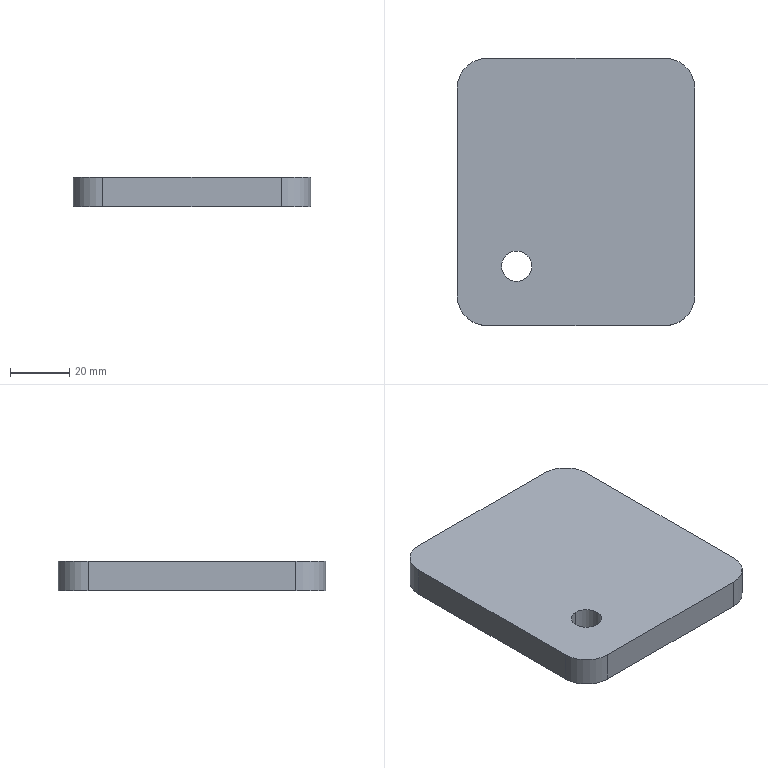Part | SolidWorks | features BaseBody 1 | 1 solid | 12 faces | box 80 x 90 x 10 mm | volume 70324 mm3 | cylinder 6 | plane 6 | commonest cylinder face diameters 20 x4 10.2 x2
STEP:
#1=CARTESIAN_POINT('',(-20.,-30.1,-5.));
#2=VERTEX_POINT('',#1);
#3=CARTESIAN_POINT('',(-20.,-19.9,-5.));
#4=VERTEX_POINT('',#3);
#5=CARTESIAN_POINT('',(-20.,-25.,-5.));
#6=DIRECTION('',(0.,0.,-1.));
#7=DIRECTION('',(0.,-1.,0.));
#8=AXIS2_PLACEMENT_3D('',#5,#6,#7);
#9=CIRCLE('',#8,5.1);
#10=EDGE_CURVE('',#2,#4,#9,.T.);
#11=ORIENTED_EDGE('',*,*,#10,.T.);
#12=CARTESIAN_POINT('',(-20.,-19.9,5.));
#13=VERTEX_POINT('',#12);
#14=CARTESIAN_POINT('',(-20.,-19.9,-5.));
#15=DIRECTION('',(0.,0.,1.));
#16=VECTOR('',#15,1000.);
#17=LINE('',#14,#16);
#18=EDGE_CURVE('',#4,#13,#17,.T.);
#19=ORIENTED_EDGE('',*,*,#18,.T.);
#20=CARTESIAN_POINT('',(-20.,-30.1,5.));
#21=VERTEX_POINT('',#20);
#22=CARTESIAN_POINT('',(-20.,-25.,5.));
#23=DIRECTION('',(0.,0.,1.));
#24=DIRECTION('',(0.,-1.,0.));
#25=AXIS2_PLACEMENT_3D('',#22,#23,#24);
#26=CIRCLE('',#25,5.1);
#27=EDGE_CURVE('',#13,#21,#26,.T.);
#28=ORIENTED_EDGE('',*,*,#27,.T.);
#29=CARTESIAN_POINT('',(-20.,-30.1,-5.));
#30=DIRECTION('',(0.,0.,1.));
#31=VECTOR('',#30,1000.);
#32=LINE('',#29,#31);
#33=EDGE_CURVE('',#2,#21,#32,.T.);
#34=ORIENTED_EDGE('',*,*,#33,.F.);
#35=EDGE_LOOP('',(#11,#19,#28,#34));
#36=FACE_OUTER_BOUND('',#35,.T.);
#37=CARTESIAN_POINT('',(-20.,-25.,-5.));
#38=DIRECTION('',(0.,0.,1.));
#39=DIRECTION('',(0.,-1.,0.));
#40=AXIS2_PLACEMENT_3D('',#37,#38,#39);
#41=CYLINDRICAL_SURFACE('',#40,5.1);
#42=ADVANCED_FACE('',(#36),#41,.F.);
#43=ORIENTED_EDGE('',*,*,#18,.F.);
#44=CARTESIAN_POINT('',(-20.,-25.,-5.));
#45=DIRECTION('',(0.,0.,-1.));
#46=DIRECTION('',(0.,-1.,0.));
#47=AXIS2_PLACEMENT_3D('',#44,#45,#46);
#48=CIRCLE('',#47,5.1);
#49=EDGE_CURVE('',#4,#2,#48,.T.);
#50=ORIENTED_EDGE('',*,*,#49,.T.);
#51=ORIENTED_EDGE('',*,*,#33,.T.);
#52=CARTESIAN_POINT('',(-20.,-25.,5.));
#53=DIRECTION('',(0.,0.,1.));
#54=DIRECTION('',(0.,-1.,0.));
#55=AXIS2_PLACEMENT_3D('',#52,#53,#54);
#56=CIRCLE('',#55,5.1);
#57=EDGE_CURVE('',#21,#13,#56,.T.);
#58=ORIENTED_EDGE('',*,*,#57,.T.);
#59=EDGE_LOOP('',(#43,#50,#51,#58));
#60=FACE_OUTER_BOUND('',#59,.T.);
#61=CARTESIAN_POINT('',(-20.,-25.,-5.));
#62=DIRECTION('',(0.,0.,1.));
#63=DIRECTION('',(0.,-1.,0.));
#64=AXIS2_PLACEMENT_3D('',#61,#62,#63);
#65=CYLINDRICAL_SURFACE('',#64,5.1);
#66=ADVANCED_FACE('',(#60),#65,.F.);
#67=ORIENTED_EDGE('',*,*,#57,.F.);
#68=ORIENTED_EDGE('',*,*,#27,.F.);
#69=EDGE_LOOP('',(#67,#68));
#70=FACE_BOUND('',#69,.T.);
#71=CARTESIAN_POINT('',(40.,-35.,5.));
#72=VERTEX_POINT('',#71);
#73=CARTESIAN_POINT('',(30.,-45.,5.));
#74=VERTEX_POINT('',#73);
#75=CARTESIAN_POINT('',(30.,-35.,5.));
#76=DIRECTION('',(0.,0.,-1.));
#77=DIRECTION('',(0.,1.,0.));
#78=AXIS2_PLACEMENT_3D('',#75,#76,#77);
#79=CIRCLE('',#78,10.);
#80=EDGE_CURVE('',#72,#74,#79,.T.);
#81=ORIENTED_EDGE('',*,*,#80,.F.);
#82=CARTESIAN_POINT('',(40.,35.,5.));
#83=VERTEX_POINT('',#82);
#84=CARTESIAN_POINT('',(40.,0.,5.));
#85=DIRECTION('',(0.,-1.,0.));
#86=VECTOR('',#85,1000.);
#87=LINE('',#84,#86);
#88=EDGE_CURVE('',#83,#72,#87,.T.);
#89=ORIENTED_EDGE('',*,*,#88,.F.);
#90=CARTESIAN_POINT('',(30.,45.,5.));
#91=VERTEX_POINT('',#90);
#92=CARTESIAN_POINT('',(30.,35.,5.));
#93=DIRECTION('',(0.,0.,-1.));
#94=DIRECTION('',(0.,1.,0.));
#95=AXIS2_PLACEMENT_3D('',#92,#93,#94);
#96=CIRCLE('',#95,10.);
#97=EDGE_CURVE('',#91,#83,#96,.T.);
#98=ORIENTED_EDGE('',*,*,#97,.F.);
#99=CARTESIAN_POINT('',(-30.,45.,5.));
#100=VERTEX_POINT('',#99);
#101=CARTESIAN_POINT('',(0.,45.,5.));
#102=DIRECTION('',(1.,0.,0.));
#103=VECTOR('',#102,1000.);
#104=LINE('',#101,#103);
#105=EDGE_CURVE('',#100,#91,#104,.T.);
#106=ORIENTED_EDGE('',*,*,#105,.F.);
#107=CARTESIAN_POINT('',(-40.,35.,5.));
#108=VERTEX_POINT('',#107);
#109=CARTESIAN_POINT('',(-30.,35.,5.));
#110=DIRECTION('',(0.,0.,-1.));
#111=DIRECTION('',(0.,1.,0.));
#112=AXIS2_PLACEMENT_3D('',#109,#110,#111);
#113=CIRCLE('',#112,10.);
#114=EDGE_CURVE('',#108,#100,#113,.T.);
#115=ORIENTED_EDGE('',*,*,#114,.F.);
#116=CARTESIAN_POINT('',(-40.,-35.,5.));
#117=VERTEX_POINT('',#116);
#118=CARTESIAN_POINT('',(-40.,0.,5.));
#119=DIRECTION('',(0.,1.,0.));
#120=VECTOR('',#119,1000.);
#121=LINE('',#118,#120);
#122=EDGE_CURVE('',#117,#108,#121,.T.);
#123=ORIENTED_EDGE('',*,*,#122,.F.);
#124=CARTESIAN_POINT('',(-30.,-45.,5.));
#125=VERTEX_POINT('',#124);
#126=CARTESIAN_POINT('',(-30.,-35.,5.));
#127=DIRECTION('',(0.,0.,-1.));
#128=DIRECTION('',(0.,1.,0.));
#129=AXIS2_PLACEMENT_3D('',#126,#127,#128);
#130=CIRCLE('',#129,10.);
#131=EDGE_CURVE('',#125,#117,#130,.T.);
#132=ORIENTED_EDGE('',*,*,#131,.F.);
#133=CARTESIAN_POINT('',(0.,-45.,5.));
#134=DIRECTION('',(-1.,0.,0.));
#135=VECTOR('',#134,1000.);
#136=LINE('',#133,#135);
#137=EDGE_CURVE('',#74,#125,#136,.T.);
#138=ORIENTED_EDGE('',*,*,#137,.F.);
#139=EDGE_LOOP('',(#81,#89,#98,#106,#115,#123,#132,#138));
#140=FACE_OUTER_BOUND('',#139,.T.);
#141=CARTESIAN_POINT('',(40.,-45.,5.));
#142=DIRECTION('',(0.,0.,-1.));
#143=DIRECTION('',(-1.,0.,0.));
#144=AXIS2_PLACEMENT_3D('',#141,#142,#143);
#145=PLANE('',#144);
#146=ADVANCED_FACE('',(#70,#140),#145,.F.);
#147=ORIENTED_EDGE('',*,*,#10,.F.);
#148=ORIENTED_EDGE('',*,*,#49,.F.);
#149=EDGE_LOOP('',(#147,#148));
#150=FACE_BOUND('',#149,.T.);
#151=CARTESIAN_POINT('',(-30.,45.,-5.));
#152=VERTEX_POINT('',#151);
#153=CARTESIAN_POINT('',(30.,45.,-5.));
#154=VERTEX_POINT('',#153);
#155=CARTESIAN_POINT('',(0.,45.,-5.));
#156=DIRECTION('',(1.,0.,0.));
#157=VECTOR('',#156,1000.);
#158=LINE('',#155,#157);
#159=EDGE_CURVE('',#152,#154,#158,.T.);
#160=ORIENTED_EDGE('',*,*,#159,.T.);
#161=CARTESIAN_POINT('',(40.,35.,-5.));
#162=VERTEX_POINT('',#161);
#163=CARTESIAN_POINT('',(30.,35.,-5.));
#164=DIRECTION('',(0.,0.,-1.));
#165=DIRECTION('',(0.,1.,0.));
#166=AXIS2_PLACEMENT_3D('',#163,#164,#165);
#167=CIRCLE('',#166,10.);
#168=EDGE_CURVE('',#154,#162,#167,.T.);
#169=ORIENTED_EDGE('',*,*,#168,.T.);
#170=CARTESIAN_POINT('',(40.,-35.,-5.));
#171=VERTEX_POINT('',#170);
#172=CARTESIAN_POINT('',(40.,0.,-5.));
#173=DIRECTION('',(0.,-1.,0.));
#174=VECTOR('',#173,1000.);
#175=LINE('',#172,#174);
#176=EDGE_CURVE('',#162,#171,#175,.T.);
#177=ORIENTED_EDGE('',*,*,#176,.T.);
#178=CARTESIAN_POINT('',(30.,-45.,-5.));
#179=VERTEX_POINT('',#178);
#180=CARTESIAN_POINT('',(30.,-35.,-5.));
#181=DIRECTION('',(0.,0.,-1.));
#182=DIRECTION('',(0.,1.,0.));
#183=AXIS2_PLACEMENT_3D('',#180,#181,#182);
#184=CIRCLE('',#183,10.);
#185=EDGE_CURVE('',#171,#179,#184,.T.);
#186=ORIENTED_EDGE('',*,*,#185,.T.);
#187=CARTESIAN_POINT('',(-30.,-45.,-5.));
#188=VERTEX_POINT('',#187);
#189=CARTESIAN_POINT('',(0.,-45.,-5.));
#190=DIRECTION('',(-1.,0.,0.));
#191=VECTOR('',#190,1000.);
#192=LINE('',#189,#191);
#193=EDGE_CURVE('',#179,#188,#192,.T.);
#194=ORIENTED_EDGE('',*,*,#193,.T.);
#195=CARTESIAN_POINT('',(-40.,-35.,-5.));
#196=VERTEX_POINT('',#195);
#197=CARTESIAN_POINT('',(-30.,-35.,-5.));
#198=DIRECTION('',(0.,0.,-1.));
#199=DIRECTION('',(0.,1.,0.));
#200=AXIS2_PLACEMENT_3D('',#197,#198,#199);
#201=CIRCLE('',#200,10.);
#202=EDGE_CURVE('',#188,#196,#201,.T.);
#203=ORIENTED_EDGE('',*,*,#202,.T.);
#204=CARTESIAN_POINT('',(-40.,35.,-5.));
#205=VERTEX_POINT('',#204);
#206=CARTESIAN_POINT('',(-40.,0.,-5.));
#207=DIRECTION('',(0.,1.,0.));
#208=VECTOR('',#207,1000.);
#209=LINE('',#206,#208);
#210=EDGE_CURVE('',#196,#205,#209,.T.);
#211=ORIENTED_EDGE('',*,*,#210,.T.);
#212=CARTESIAN_POINT('',(-30.,35.,-5.));
#213=DIRECTION('',(0.,0.,-1.));
#214=DIRECTION('',(0.,1.,0.));
#215=AXIS2_PLACEMENT_3D('',#212,#213,#214);
#216=CIRCLE('',#215,10.);
#217=EDGE_CURVE('',#205,#152,#216,.T.);
#218=ORIENTED_EDGE('',*,*,#217,.T.);
#219=EDGE_LOOP('',(#160,#169,#177,#186,#194,#203,#211,#218));
#220=FACE_OUTER_BOUND('',#219,.T.);
#221=CARTESIAN_POINT('',(40.,-45.,-5.));
#222=DIRECTION('',(0.,0.,-1.));
#223=DIRECTION('',(-1.,0.,0.));
#224=AXIS2_PLACEMENT_3D('',#221,#222,#223);
#225=PLANE('',#224);
#226=ADVANCED_FACE('',(#150,#220),#225,.T.);
#227=CARTESIAN_POINT('',(30.,-45.,0.));
#228=DIRECTION('',(0.,0.,-1.));
#229=VECTOR('',#228,1000.);
#230=LINE('',#227,#229);
#231=EDGE_CURVE('',#74,#179,#230,.T.);
#232=ORIENTED_EDGE('',*,*,#231,.F.);
#233=ORIENTED_EDGE('',*,*,#137,.T.);
#234=CARTESIAN_POINT('',(-30.,-45.,0.));
#235=DIRECTION('',(0.,0.,1.));
#236=VECTOR('',#235,1000.);
#237=LINE('',#234,#236);
#238=EDGE_CURVE('',#188,#125,#237,.T.);
#239=ORIENTED_EDGE('',*,*,#238,.F.);
#240=ORIENTED_EDGE('',*,*,#193,.F.);
#241=EDGE_LOOP('',(#232,#233,#239,#240));
#242=FACE_OUTER_BOUND('',#241,.T.);
#243=CARTESIAN_POINT('',(-30.,-45.,-5.));
#244=DIRECTION('',(0.,1.,0.));
#245=DIRECTION('',(0.,0.,1.));
#246=AXIS2_PLACEMENT_3D('',#243,#244,#245);
#247=PLANE('',#246);
#248=ADVANCED_FACE('',(#242),#247,.F.);
#249=ORIENTED_EDGE('',*,*,#231,.T.);
#250=ORIENTED_EDGE('',*,*,#185,.F.);
#251=CARTESIAN_POINT('',(40.,-35.,0.));
#252=DIRECTION('',(0.,0.,-1.));
#253=VECTOR('',#252,1000.);
#254=LINE('',#251,#253);
#255=EDGE_CURVE('',#72,#171,#254,.T.);
#256=ORIENTED_EDGE('',*,*,#255,.F.);
#257=ORIENTED_EDGE('',*,*,#80,.T.);
#258=EDGE_LOOP('',(#249,#250,#256,#257));
#259=FACE_OUTER_BOUND('',#258,.T.);
#260=CARTESIAN_POINT('',(30.,-35.,5.));
#261=DIRECTION('',(0.,0.,-1.));
#262=DIRECTION('',(0.,1.,0.));
#263=AXIS2_PLACEMENT_3D('',#260,#261,#262);
#264=CYLINDRICAL_SURFACE('',#263,10.);
#265=ADVANCED_FACE('',(#259),#264,.T.);
#266=ORIENTED_EDGE('',*,*,#255,.T.);
#267=ORIENTED_EDGE('',*,*,#176,.F.);
#268=CARTESIAN_POINT('',(40.,35.,0.));
#269=DIRECTION('',(0.,0.,-1.));
#270=VECTOR('',#269,1000.);
#271=LINE('',#268,#270);
#272=EDGE_CURVE('',#83,#162,#271,.T.);
#273=ORIENTED_EDGE('',*,*,#272,.F.);
#274=ORIENTED_EDGE('',*,*,#88,.T.);
#275=EDGE_LOOP('',(#266,#267,#273,#274));
#276=FACE_OUTER_BOUND('',#275,.T.);
#277=CARTESIAN_POINT('',(40.,-35.,-5.));
#278=DIRECTION('',(-1.,0.,0.));
#279=DIRECTION('',(0.,0.,1.));
#280=AXIS2_PLACEMENT_3D('',#277,#278,#279);
#281=PLANE('',#280);
#282=ADVANCED_FACE('',(#276),#281,.F.);
#283=ORIENTED_EDGE('',*,*,#272,.T.);
#284=ORIENTED_EDGE('',*,*,#168,.F.);
#285=CARTESIAN_POINT('',(30.,45.,0.));
#286=DIRECTION('',(0.,0.,-1.));
#287=VECTOR('',#286,1000.);
#288=LINE('',#285,#287);
#289=EDGE_CURVE('',#91,#154,#288,.T.);
#290=ORIENTED_EDGE('',*,*,#289,.F.);
#291=ORIENTED_EDGE('',*,*,#97,.T.);
#292=EDGE_LOOP('',(#283,#284,#290,#291));
#293=FACE_OUTER_BOUND('',#292,.T.);
#294=CARTESIAN_POINT('',(30.,35.,5.));
#295=DIRECTION('',(0.,0.,-1.));
#296=DIRECTION('',(0.,1.,0.));
#297=AXIS2_PLACEMENT_3D('',#294,#295,#296);
#298=CYLINDRICAL_SURFACE('',#297,10.);
#299=ADVANCED_FACE('',(#293),#298,.T.);
#300=ORIENTED_EDGE('',*,*,#289,.T.);
#301=ORIENTED_EDGE('',*,*,#159,.F.);
#302=CARTESIAN_POINT('',(-30.,45.,0.));
#303=DIRECTION('',(0.,0.,-1.));
#304=VECTOR('',#303,1000.);
#305=LINE('',#302,#304);
#306=EDGE_CURVE('',#100,#152,#305,.T.);
#307=ORIENTED_EDGE('',*,*,#306,.F.);
#308=ORIENTED_EDGE('',*,*,#105,.T.);
#309=EDGE_LOOP('',(#300,#301,#307,#308));
#310=FACE_OUTER_BOUND('',#309,.T.);
#311=CARTESIAN_POINT('',(-30.,45.,5.));
#312=DIRECTION('',(0.,-1.,0.));
#313=DIRECTION('',(0.,0.,-1.));
#314=AXIS2_PLACEMENT_3D('',#311,#312,#313);
#315=PLANE('',#314);
#316=ADVANCED_FACE('',(#310),#315,.F.);
#317=ORIENTED_EDGE('',*,*,#306,.T.);
#318=ORIENTED_EDGE('',*,*,#217,.F.);
#319=CARTESIAN_POINT('',(-40.,35.,0.));
#320=DIRECTION('',(0.,0.,-1.));
#321=VECTOR('',#320,1000.);
#322=LINE('',#319,#321);
#323=EDGE_CURVE('',#108,#205,#322,.T.);
#324=ORIENTED_EDGE('',*,*,#323,.F.);
#325=ORIENTED_EDGE('',*,*,#114,.T.);
#326=EDGE_LOOP('',(#317,#318,#324,#325));
#327=FACE_OUTER_BOUND('',#326,.T.);
#328=CARTESIAN_POINT('',(-30.,35.,5.));
#329=DIRECTION('',(0.,0.,-1.));
#330=DIRECTION('',(0.,1.,0.));
#331=AXIS2_PLACEMENT_3D('',#328,#329,#330);
#332=CYLINDRICAL_SURFACE('',#331,10.);
#333=ADVANCED_FACE('',(#327),#332,.T.);
#334=CARTESIAN_POINT('',(-40.,-35.,0.));
#335=DIRECTION('',(0.,0.,-1.));
#336=VECTOR('',#335,1000.);
#337=LINE('',#334,#336);
#338=EDGE_CURVE('',#117,#196,#337,.T.);
#339=ORIENTED_EDGE('',*,*,#338,.F.);
#340=ORIENTED_EDGE('',*,*,#122,.T.);
#341=ORIENTED_EDGE('',*,*,#323,.T.);
#342=ORIENTED_EDGE('',*,*,#210,.F.);
#343=EDGE_LOOP('',(#339,#340,#341,#342));
#344=FACE_OUTER_BOUND('',#343,.T.);
#345=CARTESIAN_POINT('',(-40.,-35.,5.));
#346=DIRECTION('',(1.,0.,0.));
#347=DIRECTION('',(0.,0.,-1.));
#348=AXIS2_PLACEMENT_3D('',#345,#346,#347);
#349=PLANE('',#348);
#350=ADVANCED_FACE('',(#344),#349,.F.);
#351=ORIENTED_EDGE('',*,*,#338,.T.);
#352=ORIENTED_EDGE('',*,*,#202,.F.);
#353=ORIENTED_EDGE('',*,*,#238,.T.);
#354=ORIENTED_EDGE('',*,*,#131,.T.);
#355=EDGE_LOOP('',(#351,#352,#353,#354));
#356=FACE_OUTER_BOUND('',#355,.T.);
#357=CARTESIAN_POINT('',(-30.,-35.,5.));
#358=DIRECTION('',(0.,0.,-1.));
#359=DIRECTION('',(0.,1.,0.));
#360=AXIS2_PLACEMENT_3D('',#357,#358,#359);
#361=CYLINDRICAL_SURFACE('',#360,10.);
#362=ADVANCED_FACE('',(#356),#361,.T.);
#363=CLOSED_SHELL('',(#42,#66,#146,#226,#248,#265,#282,#299,#316,#333,#350,#362));
#364=MANIFOLD_SOLID_BREP('',#363);
#365=CARTESIAN_POINT('',(0.,0.,0.));
#366=DIRECTION('',(0.,0.,1.));
#367=DIRECTION('',(1.,0.,0.));
#368=AXIS2_PLACEMENT_3D('',#365,#366,#367);
#369=(LENGTH_UNIT()NAMED_UNIT(*)SI_UNIT(.MILLI.,.METRE.));
#370=UNCERTAINTY_MEASURE_WITH_UNIT(LENGTH_MEASURE(0.00001),#369,'','');
#371=(NAMED_UNIT(*)PLANE_ANGLE_UNIT()SI_UNIT($,.RADIAN.));
#372=(NAMED_UNIT(*)SI_UNIT($,.STERADIAN.)SOLID_ANGLE_UNIT());
#373=(GEOMETRIC_REPRESENTATION_CONTEXT(3)GLOBAL_UNCERTAINTY_ASSIGNED_CONTEXT((#370))GLOBAL_UNIT_ASSIGNED_CONTEXT((#369,#371,#372))REPRESENTATION_CONTEXT('',''));
#374=ADVANCED_BREP_SHAPE_REPRESENTATION('',(#364,#368),#373);